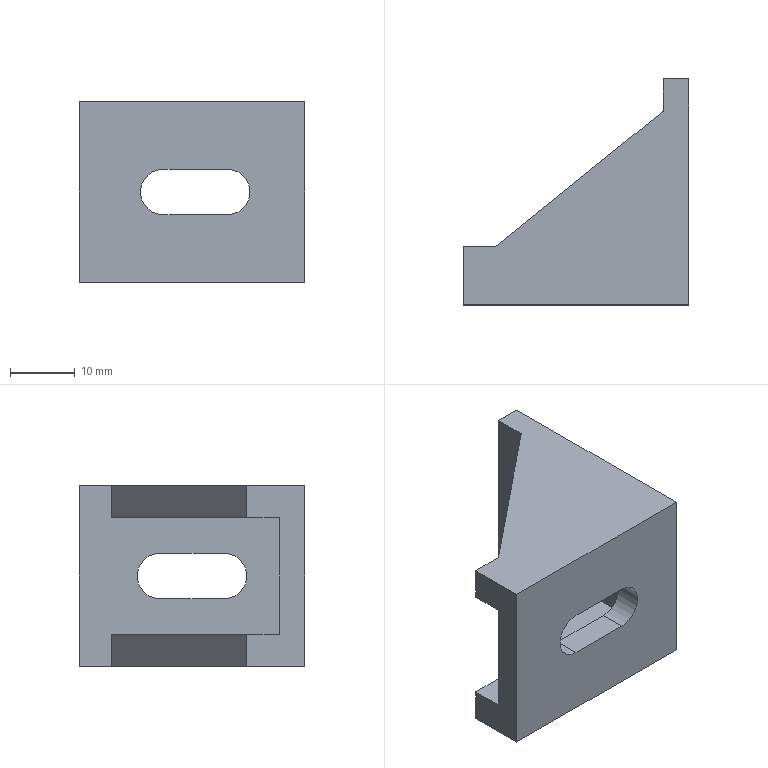Part | SolidWorks | features ICE 3, Extrusion 1, MirrorPattern 1 | 1 solid | 22 faces | box 35 x 35 x 28 mm | volume 10804 mm3 | plane 18 | cylinder 4 | commonest cylinder face diameters 7 x4
STEP:
#1=CARTESIAN_POINT('',(-2.,-5.,-3.5));
#2=VERTEX_POINT('',#1);
#3=CARTESIAN_POINT('',(-2.,-5.,3.5));
#4=VERTEX_POINT('',#3);
#5=CARTESIAN_POINT('',(-2.,-5.,0.));
#6=DIRECTION('',(-1.,0.,0.));
#7=DIRECTION('',(0.,0.,1.));
#8=AXIS2_PLACEMENT_3D('',#5,#6,#7);
#9=CIRCLE('',#8,3.5);
#10=EDGE_CURVE('',#2,#4,#9,.T.);
#11=ORIENTED_EDGE('',*,*,#10,.F.);
#12=CARTESIAN_POINT('',(-2.,5.,-3.5));
#13=VERTEX_POINT('',#12);
#14=CARTESIAN_POINT('',(-2.,-5.,-3.5));
#15=DIRECTION('',(0.,-1.,0.));
#16=VECTOR('',#15,1000.);
#17=LINE('',#14,#16);
#18=EDGE_CURVE('',#13,#2,#17,.T.);
#19=ORIENTED_EDGE('',*,*,#18,.F.);
#20=CARTESIAN_POINT('',(-2.,5.,3.5));
#21=VERTEX_POINT('',#20);
#22=CARTESIAN_POINT('',(-2.,5.,0.));
#23=DIRECTION('',(-1.,0.,0.));
#24=DIRECTION('',(0.,0.,1.));
#25=AXIS2_PLACEMENT_3D('',#22,#23,#24);
#26=CIRCLE('',#25,3.5);
#27=EDGE_CURVE('',#21,#13,#26,.T.);
#28=ORIENTED_EDGE('',*,*,#27,.F.);
#29=CARTESIAN_POINT('',(-2.,-5.,3.5));
#30=DIRECTION('',(0.,1.,0.));
#31=VECTOR('',#30,1000.);
#32=LINE('',#29,#31);
#33=EDGE_CURVE('',#4,#21,#32,.T.);
#34=ORIENTED_EDGE('',*,*,#33,.F.);
#35=EDGE_LOOP('',(#11,#19,#28,#34));
#36=FACE_BOUND('',#35,.T.);
#37=CARTESIAN_POINT('',(-2.,12.5,9.));
#38=VERTEX_POINT('',#37);
#39=CARTESIAN_POINT('',(-2.,-13.5,9.));
#40=VERTEX_POINT('',#39);
#41=CARTESIAN_POINT('',(-2.,-13.5,9.));
#42=DIRECTION('',(0.,-1.,0.));
#43=VECTOR('',#42,1000.);
#44=LINE('',#41,#43);
#45=EDGE_CURVE('',#38,#40,#44,.T.);
#46=ORIENTED_EDGE('',*,*,#45,.F.);
#47=CARTESIAN_POINT('',(-2.,12.5,14.));
#48=VERTEX_POINT('',#47);
#49=CARTESIAN_POINT('',(-2.,12.5,9.));
#50=DIRECTION('',(0.,0.,1.));
#51=VECTOR('',#50,1000.);
#52=LINE('',#49,#51);
#53=EDGE_CURVE('',#38,#48,#52,.T.);
#54=ORIENTED_EDGE('',*,*,#53,.T.);
#55=CARTESIAN_POINT('',(-2.,17.5,14.));
#56=VERTEX_POINT('',#55);
#57=CARTESIAN_POINT('',(-2.,0.,14.));
#58=DIRECTION('',(0.,1.,0.));
#59=VECTOR('',#58,1000.);
#60=LINE('',#57,#59);
#61=EDGE_CURVE('',#48,#56,#60,.T.);
#62=ORIENTED_EDGE('',*,*,#61,.T.);
#63=CARTESIAN_POINT('',(-2.,17.5,-14.));
#64=VERTEX_POINT('',#63);
#65=CARTESIAN_POINT('',(-2.,17.5,14.));
#66=DIRECTION('',(0.,0.,-1.));
#67=VECTOR('',#66,1000.);
#68=LINE('',#65,#67);
#69=EDGE_CURVE('',#56,#64,#68,.T.);
#70=ORIENTED_EDGE('',*,*,#69,.T.);
#71=CARTESIAN_POINT('',(-2.,12.5,-14.));
#72=VERTEX_POINT('',#71);
#73=CARTESIAN_POINT('',(-2.,0.,-14.));
#74=DIRECTION('',(0.,1.,0.));
#75=VECTOR('',#74,1000.);
#76=LINE('',#73,#75);
#77=EDGE_CURVE('',#72,#64,#76,.T.);
#78=ORIENTED_EDGE('',*,*,#77,.F.);
#79=CARTESIAN_POINT('',(-2.,12.5,-9.));
#80=VERTEX_POINT('',#79);
#81=CARTESIAN_POINT('',(-2.,12.5,-9.));
#82=DIRECTION('',(0.,0.,-1.));
#83=VECTOR('',#82,1000.);
#84=LINE('',#81,#83);
#85=EDGE_CURVE('',#80,#72,#84,.T.);
#86=ORIENTED_EDGE('',*,*,#85,.F.);
#87=CARTESIAN_POINT('',(-2.,-13.5,-9.));
#88=VERTEX_POINT('',#87);
#89=CARTESIAN_POINT('',(-2.,-13.5,-9.));
#90=DIRECTION('',(0.,-1.,0.));
#91=VECTOR('',#90,1000.);
#92=LINE('',#89,#91);
#93=EDGE_CURVE('',#80,#88,#92,.T.);
#94=ORIENTED_EDGE('',*,*,#93,.T.);
#95=CARTESIAN_POINT('',(-2.,-13.5,14.));
#96=DIRECTION('',(0.,0.,-1.));
#97=VECTOR('',#96,1000.);
#98=LINE('',#95,#97);
#99=EDGE_CURVE('',#40,#88,#98,.T.);
#100=ORIENTED_EDGE('',*,*,#99,.F.);
#101=EDGE_LOOP('',(#46,#54,#62,#70,#78,#86,#94,#100));
#102=FACE_OUTER_BOUND('',#101,.T.);
#103=CARTESIAN_POINT('',(-2.,0.,14.));
#104=DIRECTION('',(-1.,0.,0.));
#105=DIRECTION('',(0.,0.,1.));
#106=AXIS2_PLACEMENT_3D('',#103,#104,#105);
#107=PLANE('',#106);
#108=ADVANCED_FACE('',(#36,#102),#107,.T.);
#109=CARTESIAN_POINT('',(-20.,-13.5,-3.5));
#110=VERTEX_POINT('',#109);
#111=CARTESIAN_POINT('',(-20.,-13.5,3.5));
#112=VERTEX_POINT('',#111);
#113=CARTESIAN_POINT('',(-20.,-13.5,0.));
#114=DIRECTION('',(0.,1.,0.));
#115=DIRECTION('',(0.,0.,1.));
#116=AXIS2_PLACEMENT_3D('',#113,#114,#115);
#117=CIRCLE('',#116,3.5);
#118=EDGE_CURVE('',#110,#112,#117,.T.);
#119=ORIENTED_EDGE('',*,*,#118,.F.);
#120=CARTESIAN_POINT('',(-10.,-13.5,-3.5));
#121=VERTEX_POINT('',#120);
#122=CARTESIAN_POINT('',(-20.,-13.5,-3.5));
#123=DIRECTION('',(-1.,0.,0.));
#124=VECTOR('',#123,1000.);
#125=LINE('',#122,#124);
#126=EDGE_CURVE('',#121,#110,#125,.T.);
#127=ORIENTED_EDGE('',*,*,#126,.F.);
#128=CARTESIAN_POINT('',(-10.,-13.5,3.5));
#129=VERTEX_POINT('',#128);
#130=CARTESIAN_POINT('',(-10.,-13.5,0.));
#131=DIRECTION('',(0.,1.,0.));
#132=DIRECTION('',(0.,0.,1.));
#133=AXIS2_PLACEMENT_3D('',#130,#131,#132);
#134=CIRCLE('',#133,3.5);
#135=EDGE_CURVE('',#129,#121,#134,.T.);
#136=ORIENTED_EDGE('',*,*,#135,.F.);
#137=CARTESIAN_POINT('',(-20.,-13.5,3.5));
#138=DIRECTION('',(1.,0.,0.));
#139=VECTOR('',#138,1000.);
#140=LINE('',#137,#139);
#141=EDGE_CURVE('',#112,#129,#140,.T.);
#142=ORIENTED_EDGE('',*,*,#141,.F.);
#143=EDGE_LOOP('',(#119,#127,#136,#142));
#144=FACE_BOUND('',#143,.T.);
#145=CARTESIAN_POINT('',(-33.,-13.5,9.));
#146=VERTEX_POINT('',#145);
#147=CARTESIAN_POINT('',(-33.,-13.5,9.));
#148=DIRECTION('',(-1.,0.,0.));
#149=VECTOR('',#148,1000.);
#150=LINE('',#147,#149);
#151=EDGE_CURVE('',#40,#146,#150,.T.);
#152=ORIENTED_EDGE('',*,*,#151,.F.);
#153=ORIENTED_EDGE('',*,*,#99,.T.);
#154=CARTESIAN_POINT('',(-33.,-13.5,-9.));
#155=VERTEX_POINT('',#154);
#156=CARTESIAN_POINT('',(-33.,-13.5,-9.));
#157=DIRECTION('',(-1.,0.,0.));
#158=VECTOR('',#157,1000.);
#159=LINE('',#156,#158);
#160=EDGE_CURVE('',#88,#155,#159,.T.);
#161=ORIENTED_EDGE('',*,*,#160,.T.);
#162=CARTESIAN_POINT('',(-33.,-13.5,14.));
#163=DIRECTION('',(0.,0.,-1.));
#164=VECTOR('',#163,1000.);
#165=LINE('',#162,#164);
#166=EDGE_CURVE('',#146,#155,#165,.T.);
#167=ORIENTED_EDGE('',*,*,#166,.F.);
#168=EDGE_LOOP('',(#152,#153,#161,#167));
#169=FACE_OUTER_BOUND('',#168,.T.);
#170=CARTESIAN_POINT('',(0.,-13.5,14.));
#171=DIRECTION('',(0.,1.,0.));
#172=DIRECTION('',(0.,0.,1.));
#173=AXIS2_PLACEMENT_3D('',#170,#171,#172);
#174=PLANE('',#173);
#175=ADVANCED_FACE('',(#144,#169),#174,.T.);
#176=CARTESIAN_POINT('',(-33.,-8.5,-14.));
#177=VERTEX_POINT('',#176);
#178=CARTESIAN_POINT('',(-33.,-17.5,-14.));
#179=VERTEX_POINT('',#178);
#180=CARTESIAN_POINT('',(-33.,0.,-14.));
#181=DIRECTION('',(0.,-1.,0.));
#182=VECTOR('',#181,1000.);
#183=LINE('',#180,#182);
#184=EDGE_CURVE('',#177,#179,#183,.T.);
#185=ORIENTED_EDGE('',*,*,#184,.T.);
#186=CARTESIAN_POINT('',(-33.,-17.5,14.));
#187=VERTEX_POINT('',#186);
#188=CARTESIAN_POINT('',(-33.,-17.5,14.));
#189=DIRECTION('',(0.,0.,-1.));
#190=VECTOR('',#189,1000.);
#191=LINE('',#188,#190);
#192=EDGE_CURVE('',#187,#179,#191,.T.);
#193=ORIENTED_EDGE('',*,*,#192,.F.);
#194=CARTESIAN_POINT('',(-33.,-8.5,14.));
#195=VERTEX_POINT('',#194);
#196=CARTESIAN_POINT('',(-33.,0.,14.));
#197=DIRECTION('',(0.,-1.,0.));
#198=VECTOR('',#197,1000.);
#199=LINE('',#196,#198);
#200=EDGE_CURVE('',#195,#187,#199,.T.);
#201=ORIENTED_EDGE('',*,*,#200,.F.);
#202=CARTESIAN_POINT('',(-33.,-8.5,9.));
#203=VERTEX_POINT('',#202);
#204=CARTESIAN_POINT('',(-33.,-8.5,9.));
#205=DIRECTION('',(0.,0.,1.));
#206=VECTOR('',#205,1000.);
#207=LINE('',#204,#206);
#208=EDGE_CURVE('',#203,#195,#207,.T.);
#209=ORIENTED_EDGE('',*,*,#208,.F.);
#210=CARTESIAN_POINT('',(-33.,-8.5,9.));
#211=DIRECTION('',(0.,1.,0.));
#212=VECTOR('',#211,1000.);
#213=LINE('',#210,#212);
#214=EDGE_CURVE('',#146,#203,#213,.T.);
#215=ORIENTED_EDGE('',*,*,#214,.F.);
#216=ORIENTED_EDGE('',*,*,#166,.T.);
#217=CARTESIAN_POINT('',(-33.,-8.5,-9.));
#218=VERTEX_POINT('',#217);
#219=CARTESIAN_POINT('',(-33.,-8.5,-9.));
#220=DIRECTION('',(0.,1.,0.));
#221=VECTOR('',#220,1000.);
#222=LINE('',#219,#221);
#223=EDGE_CURVE('',#155,#218,#222,.T.);
#224=ORIENTED_EDGE('',*,*,#223,.T.);
#225=CARTESIAN_POINT('',(-33.,-8.5,-9.));
#226=DIRECTION('',(0.,0.,-1.));
#227=VECTOR('',#226,1000.);
#228=LINE('',#225,#227);
#229=EDGE_CURVE('',#218,#177,#228,.T.);
#230=ORIENTED_EDGE('',*,*,#229,.T.);
#231=EDGE_LOOP('',(#185,#193,#201,#209,#215,#216,#224,#230));
#232=FACE_OUTER_BOUND('',#231,.T.);
#233=CARTESIAN_POINT('',(-33.,0.,14.));
#234=DIRECTION('',(1.,0.,0.));
#235=DIRECTION('',(0.,1.,0.));
#236=AXIS2_PLACEMENT_3D('',#233,#234,#235);
#237=PLANE('',#236);
#238=ADVANCED_FACE('',(#232),#237,.F.);
#239=CARTESIAN_POINT('',(-20.,-17.5,3.5));
#240=VERTEX_POINT('',#239);
#241=CARTESIAN_POINT('',(-20.,-17.5,-3.5));
#242=VERTEX_POINT('',#241);
#243=CARTESIAN_POINT('',(-20.,-17.5,0.));
#244=DIRECTION('',(0.,-1.,0.));
#245=DIRECTION('',(0.,0.,-1.));
#246=AXIS2_PLACEMENT_3D('',#243,#244,#245);
#247=CIRCLE('',#246,3.5);
#248=EDGE_CURVE('',#240,#242,#247,.T.);
#249=ORIENTED_EDGE('',*,*,#248,.F.);
#250=CARTESIAN_POINT('',(-10.,-17.5,3.5));
#251=VERTEX_POINT('',#250);
#252=CARTESIAN_POINT('',(0.,-17.5,3.5));
#253=DIRECTION('',(-1.,0.,0.));
#254=VECTOR('',#253,1000.);
#255=LINE('',#252,#254);
#256=EDGE_CURVE('',#251,#240,#255,.T.);
#257=ORIENTED_EDGE('',*,*,#256,.F.);
#258=CARTESIAN_POINT('',(-10.,-17.5,-3.5));
#259=VERTEX_POINT('',#258);
#260=CARTESIAN_POINT('',(-10.,-17.5,0.));
#261=DIRECTION('',(0.,-1.,0.));
#262=DIRECTION('',(0.,0.,-1.));
#263=AXIS2_PLACEMENT_3D('',#260,#261,#262);
#264=CIRCLE('',#263,3.5);
#265=EDGE_CURVE('',#259,#251,#264,.T.);
#266=ORIENTED_EDGE('',*,*,#265,.F.);
#267=CARTESIAN_POINT('',(0.,-17.5,-3.5));
#268=DIRECTION('',(1.,0.,0.));
#269=VECTOR('',#268,1000.);
#270=LINE('',#267,#269);
#271=EDGE_CURVE('',#242,#259,#270,.T.);
#272=ORIENTED_EDGE('',*,*,#271,.F.);
#273=EDGE_LOOP('',(#249,#257,#266,#272));
#274=FACE_BOUND('',#273,.T.);
#275=CARTESIAN_POINT('',(2.,-17.5,-14.));
#276=VERTEX_POINT('',#275);
#277=CARTESIAN_POINT('',(0.,-17.5,-14.));
#278=DIRECTION('',(-1.,0.,0.));
#279=VECTOR('',#278,1000.);
#280=LINE('',#277,#279);
#281=EDGE_CURVE('',#276,#179,#280,.T.);
#282=ORIENTED_EDGE('',*,*,#281,.F.);
#283=CARTESIAN_POINT('',(2.,-17.5,14.));
#284=VERTEX_POINT('',#283);
#285=CARTESIAN_POINT('',(2.,-17.5,14.));
#286=DIRECTION('',(0.,0.,-1.));
#287=VECTOR('',#286,1000.);
#288=LINE('',#285,#287);
#289=EDGE_CURVE('',#284,#276,#288,.T.);
#290=ORIENTED_EDGE('',*,*,#289,.F.);
#291=CARTESIAN_POINT('',(0.,-17.5,14.));
#292=DIRECTION('',(-1.,0.,0.));
#293=VECTOR('',#292,1000.);
#294=LINE('',#291,#293);
#295=EDGE_CURVE('',#284,#187,#294,.T.);
#296=ORIENTED_EDGE('',*,*,#295,.T.);
#297=ORIENTED_EDGE('',*,*,#192,.T.);
#298=EDGE_LOOP('',(#282,#290,#296,#297));
#299=FACE_OUTER_BOUND('',#298,.T.);
#300=CARTESIAN_POINT('',(0.,-17.5,14.));
#301=DIRECTION('',(0.,-1.,0.));
#302=DIRECTION('',(0.,0.,-1.));
#303=AXIS2_PLACEMENT_3D('',#300,#301,#302);
#304=PLANE('',#303);
#305=ADVANCED_FACE('',(#274,#299),#304,.T.);
#306=CARTESIAN_POINT('',(2.,5.,-3.5));
#307=VERTEX_POINT('',#306);
#308=CARTESIAN_POINT('',(2.,-5.,-3.5));
#309=VERTEX_POINT('',#308);
#310=CARTESIAN_POINT('',(2.,0.,-3.5));
#311=DIRECTION('',(0.,-1.,0.));
#312=VECTOR('',#311,1000.);
#313=LINE('',#310,#312);
#314=EDGE_CURVE('',#307,#309,#313,.T.);
#315=ORIENTED_EDGE('',*,*,#314,.T.);
#316=CARTESIAN_POINT('',(2.,-5.,3.5));
#317=VERTEX_POINT('',#316);
#318=CARTESIAN_POINT('',(2.,-5.,0.));
#319=DIRECTION('',(-1.,0.,0.));
#320=DIRECTION('',(0.,0.,1.));
#321=AXIS2_PLACEMENT_3D('',#318,#319,#320);
#322=CIRCLE('',#321,3.5);
#323=EDGE_CURVE('',#309,#317,#322,.T.);
#324=ORIENTED_EDGE('',*,*,#323,.T.);
#325=CARTESIAN_POINT('',(2.,5.,3.5));
#326=VERTEX_POINT('',#325);
#327=CARTESIAN_POINT('',(2.,0.,3.5));
#328=DIRECTION('',(0.,1.,0.));
#329=VECTOR('',#328,1000.);
#330=LINE('',#327,#329);
#331=EDGE_CURVE('',#317,#326,#330,.T.);
#332=ORIENTED_EDGE('',*,*,#331,.T.);
#333=CARTESIAN_POINT('',(2.,5.,0.));
#334=DIRECTION('',(-1.,0.,0.));
#335=DIRECTION('',(0.,0.,1.));
#336=AXIS2_PLACEMENT_3D('',#333,#334,#335);
#337=CIRCLE('',#336,3.5);
#338=EDGE_CURVE('',#326,#307,#337,.T.);
#339=ORIENTED_EDGE('',*,*,#338,.T.);
#340=EDGE_LOOP('',(#315,#324,#332,#339));
#341=FACE_BOUND('',#340,.T.);
#342=CARTESIAN_POINT('',(2.,17.5,-14.));
#343=VERTEX_POINT('',#342);
#344=CARTESIAN_POINT('',(2.,0.,-14.));
#345=DIRECTION('',(0.,1.,0.));
#346=VECTOR('',#345,1000.);
#347=LINE('',#344,#346);
#348=EDGE_CURVE('',#276,#343,#347,.T.);
#349=ORIENTED_EDGE('',*,*,#348,.T.);
#350=CARTESIAN_POINT('',(2.,17.5,14.));
#351=VERTEX_POINT('',#350);
#352=CARTESIAN_POINT('',(2.,17.5,14.));
#353=DIRECTION('',(0.,0.,-1.));
#354=VECTOR('',#353,1000.);
#355=LINE('',#352,#354);
#356=EDGE_CURVE('',#351,#343,#355,.T.);
#357=ORIENTED_EDGE('',*,*,#356,.F.);
#358=CARTESIAN_POINT('',(2.,0.,14.));
#359=DIRECTION('',(0.,1.,0.));
#360=VECTOR('',#359,1000.);
#361=LINE('',#358,#360);
#362=EDGE_CURVE('',#284,#351,#361,.T.);
#363=ORIENTED_EDGE('',*,*,#362,.F.);
#364=ORIENTED_EDGE('',*,*,#289,.T.);
#365=EDGE_LOOP('',(#349,#357,#363,#364));
#366=FACE_OUTER_BOUND('',#365,.T.);
#367=CARTESIAN_POINT('',(2.,0.,14.));
#368=DIRECTION('',(-1.,0.,0.));
#369=DIRECTION('',(0.,0.,1.));
#370=AXIS2_PLACEMENT_3D('',#367,#368,#369);
#371=PLANE('',#370);
#372=ADVANCED_FACE('',(#341,#366),#371,.F.);
#373=CARTESIAN_POINT('',(0.,17.5,-14.));
#374=DIRECTION('',(-1.,0.,0.));
#375=VECTOR('',#374,1000.);
#376=LINE('',#373,#375);
#377=EDGE_CURVE('',#343,#64,#376,.T.);
#378=ORIENTED_EDGE('',*,*,#377,.T.);
#379=ORIENTED_EDGE('',*,*,#69,.F.);
#380=CARTESIAN_POINT('',(0.,17.5,14.));
#381=DIRECTION('',(-1.,0.,0.));
#382=VECTOR('',#381,1000.);
#383=LINE('',#380,#382);
#384=EDGE_CURVE('',#351,#56,#383,.T.);
#385=ORIENTED_EDGE('',*,*,#384,.F.);
#386=ORIENTED_EDGE('',*,*,#356,.T.);
#387=EDGE_LOOP('',(#378,#379,#385,#386));
#388=FACE_OUTER_BOUND('',#387,.T.);
#389=CARTESIAN_POINT('',(0.,17.5,14.));
#390=DIRECTION('',(0.,-1.,0.));
#391=DIRECTION('',(0.,0.,-1.));
#392=AXIS2_PLACEMENT_3D('',#389,#390,#391);
#393=PLANE('',#392);
#394=ADVANCED_FACE('',(#388),#393,.F.);
#395=ORIENTED_EDGE('',*,*,#61,.F.);
#396=CARTESIAN_POINT('',(-28.,-8.5,14.));
#397=VERTEX_POINT('',#396);
#398=CARTESIAN_POINT('',(-2.,12.5,14.));
#399=DIRECTION('',(0.7779,0.6283,0.));
#400=VECTOR('',#399,1000.);
#401=LINE('',#398,#400);
#402=EDGE_CURVE('',#397,#48,#401,.T.);
#403=ORIENTED_EDGE('',*,*,#402,.F.);
#404=CARTESIAN_POINT('',(-28.,-8.5,14.));
#405=DIRECTION('',(1.,0.,0.));
#406=VECTOR('',#405,1000.);
#407=LINE('',#404,#406);
#408=EDGE_CURVE('',#195,#397,#407,.T.);
#409=ORIENTED_EDGE('',*,*,#408,.F.);
#410=ORIENTED_EDGE('',*,*,#200,.T.);
#411=ORIENTED_EDGE('',*,*,#295,.F.);
#412=ORIENTED_EDGE('',*,*,#362,.T.);
#413=ORIENTED_EDGE('',*,*,#384,.T.);
#414=EDGE_LOOP('',(#395,#403,#409,#410,#411,#412,#413));
#415=FACE_OUTER_BOUND('',#414,.T.);
#416=CARTESIAN_POINT('',(0.,0.,14.));
#417=DIRECTION('',(0.,0.,1.));
#418=DIRECTION('',(1.,0.,0.));
#419=AXIS2_PLACEMENT_3D('',#416,#417,#418);
#420=PLANE('',#419);
#421=ADVANCED_FACE('',(#415),#420,.T.);
#422=CARTESIAN_POINT('',(-28.,-8.5,-14.));
#423=VERTEX_POINT('',#422);
#424=CARTESIAN_POINT('',(-2.,12.5,-14.));
#425=DIRECTION('',(0.7779,0.6283,0.));
#426=VECTOR('',#425,1000.);
#427=LINE('',#424,#426);
#428=EDGE_CURVE('',#423,#72,#427,.T.);
#429=ORIENTED_EDGE('',*,*,#428,.T.);
#430=ORIENTED_EDGE('',*,*,#77,.T.);
#431=ORIENTED_EDGE('',*,*,#377,.F.);
#432=ORIENTED_EDGE('',*,*,#348,.F.);
#433=ORIENTED_EDGE('',*,*,#281,.T.);
#434=ORIENTED_EDGE('',*,*,#184,.F.);
#435=CARTESIAN_POINT('',(-28.,-8.5,-14.));
#436=DIRECTION('',(1.,0.,0.));
#437=VECTOR('',#436,1000.);
#438=LINE('',#435,#437);
#439=EDGE_CURVE('',#177,#423,#438,.T.);
#440=ORIENTED_EDGE('',*,*,#439,.T.);
#441=EDGE_LOOP('',(#429,#430,#431,#432,#433,#434,#440));
#442=FACE_OUTER_BOUND('',#441,.T.);
#443=CARTESIAN_POINT('',(0.,0.,-14.));
#444=DIRECTION('',(0.,0.,1.));
#445=DIRECTION('',(1.,0.,0.));
#446=AXIS2_PLACEMENT_3D('',#443,#444,#445);
#447=PLANE('',#446);
#448=ADVANCED_FACE('',(#442),#447,.F.);
#449=ORIENTED_EDGE('',*,*,#428,.F.);
#450=CARTESIAN_POINT('',(-28.,-8.5,-9.));
#451=VERTEX_POINT('',#450);
#452=CARTESIAN_POINT('',(-28.,-8.5,-9.));
#453=DIRECTION('',(0.,0.,-1.));
#454=VECTOR('',#453,1000.);
#455=LINE('',#452,#454);
#456=EDGE_CURVE('',#451,#423,#455,.T.);
#457=ORIENTED_EDGE('',*,*,#456,.F.);
#458=CARTESIAN_POINT('',(-2.,12.5,-9.));
#459=DIRECTION('',(0.7779,0.6283,0.));
#460=VECTOR('',#459,1000.);
#461=LINE('',#458,#460);
#462=EDGE_CURVE('',#451,#80,#461,.T.);
#463=ORIENTED_EDGE('',*,*,#462,.T.);
#464=ORIENTED_EDGE('',*,*,#85,.T.);
#465=EDGE_LOOP('',(#449,#457,#463,#464));
#466=FACE_OUTER_BOUND('',#465,.T.);
#467=CARTESIAN_POINT('',(-2.,12.5,-9.));
#468=DIRECTION('',(-0.6283,0.7779,0.));
#469=DIRECTION('',(-0.7779,-0.6283,0.));
#470=AXIS2_PLACEMENT_3D('',#467,#468,#469);
#471=PLANE('',#470);
#472=ADVANCED_FACE('',(#466),#471,.T.);
#473=ORIENTED_EDGE('',*,*,#439,.F.);
#474=ORIENTED_EDGE('',*,*,#229,.F.);
#475=CARTESIAN_POINT('',(-28.,-8.5,-9.));
#476=DIRECTION('',(1.,0.,0.));
#477=VECTOR('',#476,1000.);
#478=LINE('',#475,#477);
#479=EDGE_CURVE('',#218,#451,#478,.T.);
#480=ORIENTED_EDGE('',*,*,#479,.T.);
#481=ORIENTED_EDGE('',*,*,#456,.T.);
#482=EDGE_LOOP('',(#473,#474,#480,#481));
#483=FACE_OUTER_BOUND('',#482,.T.);
#484=CARTESIAN_POINT('',(-28.,-8.5,-9.));
#485=DIRECTION('',(0.,1.,0.));
#486=DIRECTION('',(0.,0.,1.));
#487=AXIS2_PLACEMENT_3D('',#484,#485,#486);
#488=PLANE('',#487);
#489=ADVANCED_FACE('',(#483),#488,.T.);
#490=ORIENTED_EDGE('',*,*,#93,.F.);
#491=ORIENTED_EDGE('',*,*,#462,.F.);
#492=ORIENTED_EDGE('',*,*,#479,.F.);
#493=ORIENTED_EDGE('',*,*,#223,.F.);
#494=ORIENTED_EDGE('',*,*,#160,.F.);
#495=EDGE_LOOP('',(#490,#491,#492,#493,#494));
#496=FACE_OUTER_BOUND('',#495,.T.);
#497=CARTESIAN_POINT('',(0.,0.,-9.));
#498=DIRECTION('',(0.,0.,1.));
#499=DIRECTION('',(1.,0.,0.));
#500=AXIS2_PLACEMENT_3D('',#497,#498,#499);
#501=PLANE('',#500);
#502=ADVANCED_FACE('',(#496),#501,.T.);
#503=ORIENTED_EDGE('',*,*,#408,.T.);
#504=CARTESIAN_POINT('',(-28.,-8.5,9.));
#505=VERTEX_POINT('',#504);
#506=CARTESIAN_POINT('',(-28.,-8.5,9.));
#507=DIRECTION('',(0.,0.,1.));
#508=VECTOR('',#507,1000.);
#509=LINE('',#506,#508);
#510=EDGE_CURVE('',#505,#397,#509,.T.);
#511=ORIENTED_EDGE('',*,*,#510,.F.);
#512=CARTESIAN_POINT('',(-28.,-8.5,9.));
#513=DIRECTION('',(1.,0.,0.));
#514=VECTOR('',#513,1000.);
#515=LINE('',#512,#514);
#516=EDGE_CURVE('',#203,#505,#515,.T.);
#517=ORIENTED_EDGE('',*,*,#516,.F.);
#518=ORIENTED_EDGE('',*,*,#208,.T.);
#519=EDGE_LOOP('',(#503,#511,#517,#518));
#520=FACE_OUTER_BOUND('',#519,.T.);
#521=CARTESIAN_POINT('',(-28.,-8.5,9.));
#522=DIRECTION('',(0.,-1.,0.));
#523=DIRECTION('',(0.,0.,-1.));
#524=AXIS2_PLACEMENT_3D('',#521,#522,#523);
#525=PLANE('',#524);
#526=ADVANCED_FACE('',(#520),#525,.F.);
#527=ORIENTED_EDGE('',*,*,#402,.T.);
#528=ORIENTED_EDGE('',*,*,#53,.F.);
#529=CARTESIAN_POINT('',(-2.,12.5,9.));
#530=DIRECTION('',(0.7779,0.6283,0.));
#531=VECTOR('',#530,1000.);
#532=LINE('',#529,#531);
#533=EDGE_CURVE('',#505,#38,#532,.T.);
#534=ORIENTED_EDGE('',*,*,#533,.F.);
#535=ORIENTED_EDGE('',*,*,#510,.T.);
#536=EDGE_LOOP('',(#527,#528,#534,#535));
#537=FACE_OUTER_BOUND('',#536,.T.);
#538=CARTESIAN_POINT('',(-2.,12.5,9.));
#539=DIRECTION('',(0.6283,-0.7779,0.));
#540=DIRECTION('',(0.7779,0.6283,0.));
#541=AXIS2_PLACEMENT_3D('',#538,#539,#540);
#542=PLANE('',#541);
#543=ADVANCED_FACE('',(#537),#542,.F.);
#544=ORIENTED_EDGE('',*,*,#45,.T.);
#545=ORIENTED_EDGE('',*,*,#151,.T.);
#546=ORIENTED_EDGE('',*,*,#214,.T.);
#547=ORIENTED_EDGE('',*,*,#516,.T.);
#548=ORIENTED_EDGE('',*,*,#533,.T.);
#549=EDGE_LOOP('',(#544,#545,#546,#547,#548));
#550=FACE_OUTER_BOUND('',#549,.T.);
#551=CARTESIAN_POINT('',(0.,0.,9.));
#552=DIRECTION('',(0.,0.,-1.));
#553=DIRECTION('',(1.,0.,0.));
#554=AXIS2_PLACEMENT_3D('',#551,#552,#553);
#555=PLANE('',#554);
#556=ADVANCED_FACE('',(#550),#555,.T.);
#557=CARTESIAN_POINT('',(3.,-5.,-3.5));
#558=DIRECTION('',(-1.,0.,0.));
#559=VECTOR('',#558,1000.);
#560=LINE('',#557,#559);
#561=EDGE_CURVE('',#309,#2,#560,.T.);
#562=ORIENTED_EDGE('',*,*,#561,.T.);
#563=ORIENTED_EDGE('',*,*,#10,.T.);
#564=CARTESIAN_POINT('',(3.,-5.,3.5));
#565=DIRECTION('',(-1.,0.,0.));
#566=VECTOR('',#565,1000.);
#567=LINE('',#564,#566);
#568=EDGE_CURVE('',#317,#4,#567,.T.);
#569=ORIENTED_EDGE('',*,*,#568,.F.);
#570=ORIENTED_EDGE('',*,*,#323,.F.);
#571=EDGE_LOOP('',(#562,#563,#569,#570));
#572=FACE_OUTER_BOUND('',#571,.T.);
#573=CARTESIAN_POINT('',(3.,-5.,0.));
#574=DIRECTION('',(-1.,0.,0.));
#575=DIRECTION('',(0.,0.,1.));
#576=AXIS2_PLACEMENT_3D('',#573,#574,#575);
#577=CYLINDRICAL_SURFACE('',#576,3.5);
#578=ADVANCED_FACE('',(#572),#577,.F.);
#579=CARTESIAN_POINT('',(3.,5.,-3.5));
#580=DIRECTION('',(-1.,0.,0.));
#581=VECTOR('',#580,1000.);
#582=LINE('',#579,#581);
#583=EDGE_CURVE('',#307,#13,#582,.T.);
#584=ORIENTED_EDGE('',*,*,#583,.T.);
#585=ORIENTED_EDGE('',*,*,#18,.T.);
#586=ORIENTED_EDGE('',*,*,#561,.F.);
#587=ORIENTED_EDGE('',*,*,#314,.F.);
#588=EDGE_LOOP('',(#584,#585,#586,#587));
#589=FACE_OUTER_BOUND('',#588,.T.);
#590=CARTESIAN_POINT('',(3.,-5.,-3.5));
#591=DIRECTION('',(0.,0.,-1.));
#592=DIRECTION('',(0.,1.,0.));
#593=AXIS2_PLACEMENT_3D('',#590,#591,#592);
#594=PLANE('',#593);
#595=ADVANCED_FACE('',(#589),#594,.F.);
#596=CARTESIAN_POINT('',(3.,5.,3.5));
#597=DIRECTION('',(-1.,0.,0.));
#598=VECTOR('',#597,1000.);
#599=LINE('',#596,#598);
#600=EDGE_CURVE('',#326,#21,#599,.T.);
#601=ORIENTED_EDGE('',*,*,#600,.T.);
#602=ORIENTED_EDGE('',*,*,#27,.T.);
#603=ORIENTED_EDGE('',*,*,#583,.F.);
#604=ORIENTED_EDGE('',*,*,#338,.F.);
#605=EDGE_LOOP('',(#601,#602,#603,#604));
#606=FACE_OUTER_BOUND('',#605,.T.);
#607=CARTESIAN_POINT('',(3.,5.,0.));
#608=DIRECTION('',(-1.,0.,0.));
#609=DIRECTION('',(0.,0.,1.));
#610=AXIS2_PLACEMENT_3D('',#607,#608,#609);
#611=CYLINDRICAL_SURFACE('',#610,3.5);
#612=ADVANCED_FACE('',(#606),#611,.F.);
#613=ORIENTED_EDGE('',*,*,#568,.T.);
#614=ORIENTED_EDGE('',*,*,#33,.T.);
#615=ORIENTED_EDGE('',*,*,#600,.F.);
#616=ORIENTED_EDGE('',*,*,#331,.F.);
#617=EDGE_LOOP('',(#613,#614,#615,#616));
#618=FACE_OUTER_BOUND('',#617,.T.);
#619=CARTESIAN_POINT('',(3.,-5.,3.5));
#620=DIRECTION('',(0.,0.,1.));
#621=DIRECTION('',(0.,-1.,0.));
#622=AXIS2_PLACEMENT_3D('',#619,#620,#621);
#623=PLANE('',#622);
#624=ADVANCED_FACE('',(#618),#623,.F.);
#625=ORIENTED_EDGE('',*,*,#248,.T.);
#626=CARTESIAN_POINT('',(-20.,-18.5,-3.5));
#627=DIRECTION('',(0.,1.,0.));
#628=VECTOR('',#627,1000.);
#629=LINE('',#626,#628);
#630=EDGE_CURVE('',#242,#110,#629,.T.);
#631=ORIENTED_EDGE('',*,*,#630,.T.);
#632=ORIENTED_EDGE('',*,*,#118,.T.);
#633=CARTESIAN_POINT('',(-20.,-18.5,3.5));
#634=DIRECTION('',(0.,1.,0.));
#635=VECTOR('',#634,1000.);
#636=LINE('',#633,#635);
#637=EDGE_CURVE('',#240,#112,#636,.T.);
#638=ORIENTED_EDGE('',*,*,#637,.F.);
#639=EDGE_LOOP('',(#625,#631,#632,#638));
#640=FACE_OUTER_BOUND('',#639,.T.);
#641=CARTESIAN_POINT('',(-20.,-18.5,0.));
#642=DIRECTION('',(0.,1.,0.));
#643=DIRECTION('',(0.,0.,1.));
#644=AXIS2_PLACEMENT_3D('',#641,#642,#643);
#645=CYLINDRICAL_SURFACE('',#644,3.5);
#646=ADVANCED_FACE('',(#640),#645,.F.);
#647=ORIENTED_EDGE('',*,*,#271,.T.);
#648=CARTESIAN_POINT('',(-10.,-18.5,-3.5));
#649=DIRECTION('',(0.,1.,0.));
#650=VECTOR('',#649,1000.);
#651=LINE('',#648,#650);
#652=EDGE_CURVE('',#259,#121,#651,.T.);
#653=ORIENTED_EDGE('',*,*,#652,.T.);
#654=ORIENTED_EDGE('',*,*,#126,.T.);
#655=ORIENTED_EDGE('',*,*,#630,.F.);
#656=EDGE_LOOP('',(#647,#653,#654,#655));
#657=FACE_OUTER_BOUND('',#656,.T.);
#658=CARTESIAN_POINT('',(-20.,-18.5,-3.5));
#659=DIRECTION('',(0.,0.,-1.));
#660=DIRECTION('',(-1.,0.,0.));
#661=AXIS2_PLACEMENT_3D('',#658,#659,#660);
#662=PLANE('',#661);
#663=ADVANCED_FACE('',(#657),#662,.F.);
#664=ORIENTED_EDGE('',*,*,#265,.T.);
#665=CARTESIAN_POINT('',(-10.,-18.5,3.5));
#666=DIRECTION('',(0.,1.,0.));
#667=VECTOR('',#666,1000.);
#668=LINE('',#665,#667);
#669=EDGE_CURVE('',#251,#129,#668,.T.);
#670=ORIENTED_EDGE('',*,*,#669,.T.);
#671=ORIENTED_EDGE('',*,*,#135,.T.);
#672=ORIENTED_EDGE('',*,*,#652,.F.);
#673=EDGE_LOOP('',(#664,#670,#671,#672));
#674=FACE_OUTER_BOUND('',#673,.T.);
#675=CARTESIAN_POINT('',(-10.,-18.5,0.));
#676=DIRECTION('',(0.,1.,0.));
#677=DIRECTION('',(0.,0.,1.));
#678=AXIS2_PLACEMENT_3D('',#675,#676,#677);
#679=CYLINDRICAL_SURFACE('',#678,3.5);
#680=ADVANCED_FACE('',(#674),#679,.F.);
#681=ORIENTED_EDGE('',*,*,#256,.T.);
#682=ORIENTED_EDGE('',*,*,#637,.T.);
#683=ORIENTED_EDGE('',*,*,#141,.T.);
#684=ORIENTED_EDGE('',*,*,#669,.F.);
#685=EDGE_LOOP('',(#681,#682,#683,#684));
#686=FACE_OUTER_BOUND('',#685,.T.);
#687=CARTESIAN_POINT('',(-20.,-18.5,3.5));
#688=DIRECTION('',(0.,0.,1.));
#689=DIRECTION('',(1.,0.,0.));
#690=AXIS2_PLACEMENT_3D('',#687,#688,#689);
#691=PLANE('',#690);
#692=ADVANCED_FACE('',(#686),#691,.F.);
#693=CLOSED_SHELL('',(#108,#175,#238,#305,#372,#394,#421,#448,#472,#489,#502,#526,#543,#556,#578,#595,#612,#624,#646,#663,#680,#692));
#694=MANIFOLD_SOLID_BREP('',#693);
#695=CARTESIAN_POINT('',(0.,0.,0.));
#696=DIRECTION('',(0.,0.,1.));
#697=DIRECTION('',(1.,0.,0.));
#698=AXIS2_PLACEMENT_3D('',#695,#696,#697);
#699=(LENGTH_UNIT()NAMED_UNIT(*)SI_UNIT(.MILLI.,.METRE.));
#700=UNCERTAINTY_MEASURE_WITH_UNIT(LENGTH_MEASURE(0.00001),#699,'','');
#701=(NAMED_UNIT(*)PLANE_ANGLE_UNIT()SI_UNIT($,.RADIAN.));
#702=(NAMED_UNIT(*)SI_UNIT($,.STERADIAN.)SOLID_ANGLE_UNIT());
#703=(GEOMETRIC_REPRESENTATION_CONTEXT(3)GLOBAL_UNCERTAINTY_ASSIGNED_CONTEXT((#700))GLOBAL_UNIT_ASSIGNED_CONTEXT((#699,#701,#702))REPRESENTATION_CONTEXT('',''));
#704=ADVANCED_BREP_SHAPE_REPRESENTATION('',(#694,#698),#703);